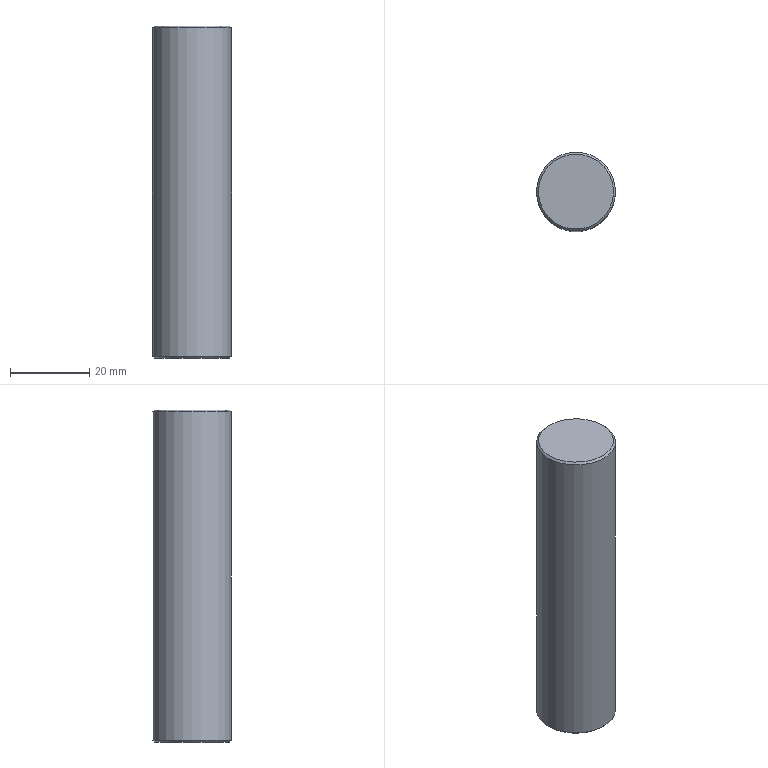Part | NX | 1 solid | 5 faces | box 20 x 20 x 84 mm | volume 26374 mm3 | plane 2 | cone 2 | cylinder 1 | commonest cylinder face diameters 20 x1
STEP:
#1=CARTESIAN_POINT('',(10.,0.,41.5));
#2=VERTEX_POINT('',#1);
#3=CARTESIAN_POINT('',(0.,0.,41.5));
#4=DIRECTION('',(0.,0.,1.));
#5=DIRECTION('',(1.,0.,0.));
#6=AXIS2_PLACEMENT_3D('',#3,#4,#5);
#7=CIRCLE('',#6,10.);
#8=EDGE_CURVE('',#2,#2,#7,.F.);
#9=ORIENTED_EDGE('',*,*,#8,.T.);
#10=EDGE_LOOP('',(#9));
#11=FACE_BOUND('',#10,.T.);
#12=CARTESIAN_POINT('',(10.,0.,-41.5));
#13=VERTEX_POINT('',#12);
#14=CARTESIAN_POINT('',(0.,0.,-41.5));
#15=DIRECTION('',(0.,0.,1.));
#16=DIRECTION('',(1.,0.,0.));
#17=AXIS2_PLACEMENT_3D('',#14,#15,#16);
#18=CIRCLE('',#17,10.);
#19=EDGE_CURVE('',#13,#13,#18,.T.);
#20=ORIENTED_EDGE('',*,*,#19,.T.);
#21=EDGE_LOOP('',(#20));
#22=FACE_BOUND('',#21,.T.);
#23=CARTESIAN_POINT('',(0.,0.,42.));
#24=DIRECTION('',(0.,0.,-1.));
#25=DIRECTION('',(-1.,0.,0.));
#26=AXIS2_PLACEMENT_3D('',#23,#24,#25);
#27=CYLINDRICAL_SURFACE('',#26,10.);
#28=ADVANCED_FACE('',(#11,#22),#27,.T.);
#29=CARTESIAN_POINT('',(9.5,0.,42.));
#30=VERTEX_POINT('',#29);
#31=CARTESIAN_POINT('',(0.,0.,42.));
#32=DIRECTION('',(0.,0.,1.));
#33=DIRECTION('',(1.,0.,0.));
#34=AXIS2_PLACEMENT_3D('',#31,#32,#33);
#35=CIRCLE('',#34,9.5);
#36=EDGE_CURVE('',#30,#30,#35,.T.);
#37=ORIENTED_EDGE('',*,*,#36,.T.);
#38=EDGE_LOOP('',(#37));
#39=FACE_BOUND('',#38,.T.);
#40=CARTESIAN_POINT('',(0.,0.,42.));
#41=DIRECTION('',(0.,0.,1.));
#42=DIRECTION('',(1.,0.,0.));
#43=AXIS2_PLACEMENT_3D('',#40,#41,#42);
#44=PLANE('',#43);
#45=ADVANCED_FACE('',(#39),#44,.T.);
#46=CARTESIAN_POINT('',(9.5,0.,-42.));
#47=VERTEX_POINT('',#46);
#48=CARTESIAN_POINT('',(0.,0.,-42.));
#49=DIRECTION('',(0.,0.,1.));
#50=DIRECTION('',(1.,0.,0.));
#51=AXIS2_PLACEMENT_3D('',#48,#49,#50);
#52=CIRCLE('',#51,9.5);
#53=EDGE_CURVE('',#47,#47,#52,.F.);
#54=ORIENTED_EDGE('',*,*,#53,.T.);
#55=EDGE_LOOP('',(#54));
#56=FACE_BOUND('',#55,.T.);
#57=CARTESIAN_POINT('',(0.,0.,-42.));
#58=DIRECTION('',(0.,0.,1.));
#59=DIRECTION('',(1.,0.,0.));
#60=AXIS2_PLACEMENT_3D('',#57,#58,#59);
#61=PLANE('',#60);
#62=ADVANCED_FACE('',(#56),#61,.F.);
#63=ORIENTED_EDGE('',*,*,#8,.F.);
#64=EDGE_LOOP('',(#63));
#65=FACE_BOUND('',#64,.T.);
#66=ORIENTED_EDGE('',*,*,#36,.F.);
#67=EDGE_LOOP('',(#66));
#68=FACE_BOUND('',#67,.T.);
#69=CARTESIAN_POINT('',(0.,0.,42.));
#70=DIRECTION('',(0.,0.,-1.));
#71=DIRECTION('',(-1.,0.,0.));
#72=AXIS2_PLACEMENT_3D('',#69,#70,#71);
#73=CONICAL_SURFACE('',#72,9.5,0.7854);
#74=ADVANCED_FACE('',(#65,#68),#73,.T.);
#75=ORIENTED_EDGE('',*,*,#53,.F.);
#76=EDGE_LOOP('',(#75));
#77=FACE_BOUND('',#76,.T.);
#78=ORIENTED_EDGE('',*,*,#19,.F.);
#79=EDGE_LOOP('',(#78));
#80=FACE_BOUND('',#79,.T.);
#81=CARTESIAN_POINT('',(0.,0.,-41.5));
#82=DIRECTION('',(0.,0.,1.));
#83=DIRECTION('',(1.,0.,0.));
#84=AXIS2_PLACEMENT_3D('',#81,#82,#83);
#85=CONICAL_SURFACE('',#84,10.,0.7854);
#86=ADVANCED_FACE('',(#77,#80),#85,.T.);
#87=CLOSED_SHELL('',(#28,#45,#62,#74,#86));
#88=MANIFOLD_SOLID_BREP('',#87);
#89=(LENGTH_UNIT()NAMED_UNIT(*)SI_UNIT(.MILLI.,.METRE.));
#90=UNCERTAINTY_MEASURE_WITH_UNIT(LENGTH_MEASURE(0.00001),#89,'','');
#91=(NAMED_UNIT(*)PLANE_ANGLE_UNIT()SI_UNIT($,.RADIAN.));
#92=(NAMED_UNIT(*)SI_UNIT($,.STERADIAN.)SOLID_ANGLE_UNIT());
#93=(GEOMETRIC_REPRESENTATION_CONTEXT(3)GLOBAL_UNCERTAINTY_ASSIGNED_CONTEXT((#90))GLOBAL_UNIT_ASSIGNED_CONTEXT((#89,#91,#92))REPRESENTATION_CONTEXT('',''));
#94=ADVANCED_BREP_SHAPE_REPRESENTATION('',(#88),#93);